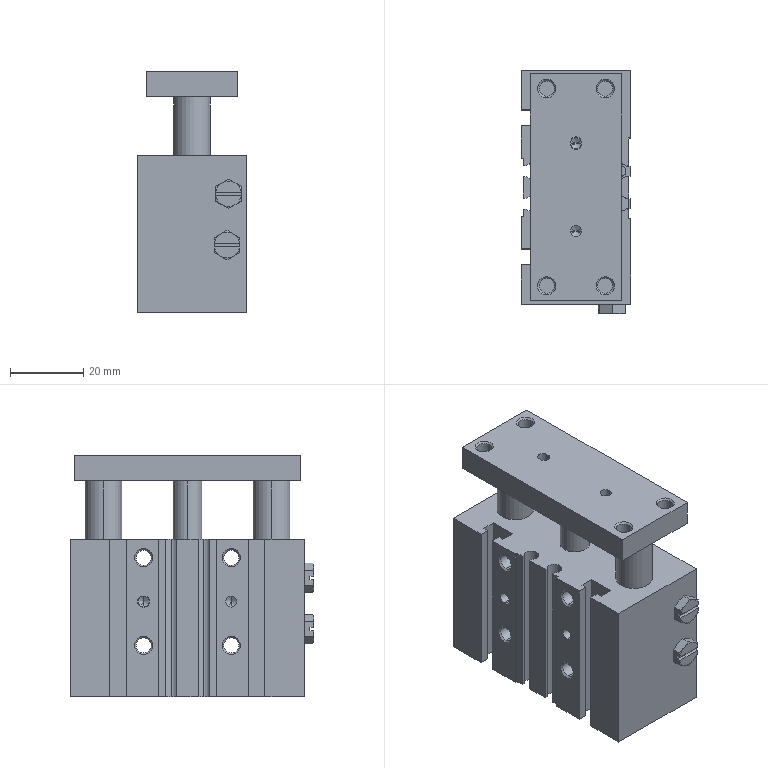Part | SolidWorks | 6 solids | 346 faces | box 30 x 66.5 x 66 mm | volume 82906 mm3 | plane 128 | cylinder 118 | cone 100 | commonest cylinder face diameters 4.134 x32 3 x18 8 x12 4.3 x8 10 x8 4 x6